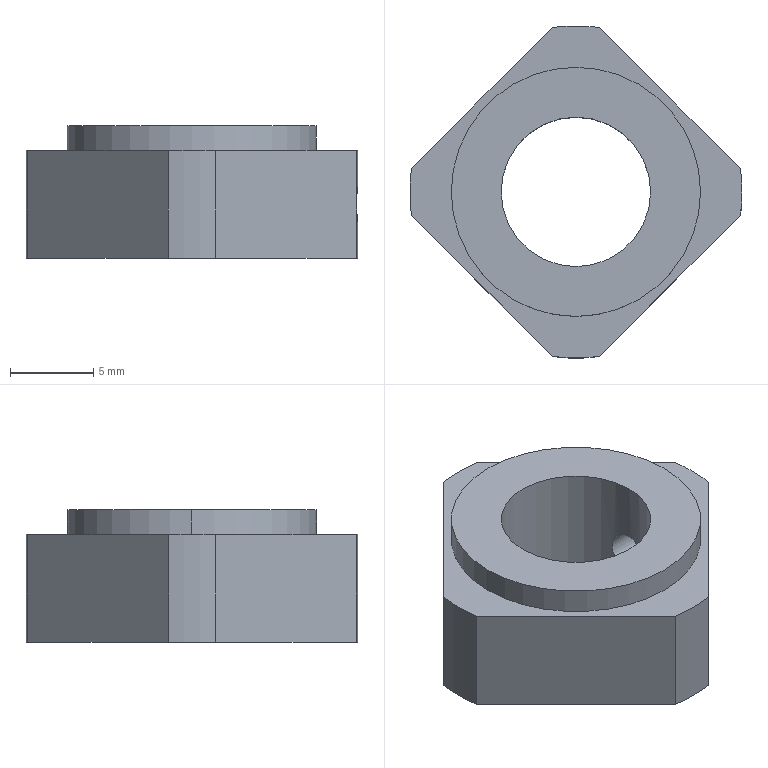Part | NX | features BREP 1 | 1 solid | 18 faces | box 20 x 20 x 8 mm | volume 1346 mm3 | cylinder 11 | plane 7 | commonest cylinder face diameters 20 x5 2.5 x2 9 x2 15 x2
STEP:
#1=CARTESIAN_POINT('',(4.5,0.,2.));
#2=VERTEX_POINT('',#1);
#3=CARTESIAN_POINT('',(10.,0.,2.));
#4=VERTEX_POINT('',#3);
#5=CARTESIAN_POINT('',(0.,0.,2.));
#6=DIRECTION('',(-1.,0.,0.));
#7=VECTOR('',#6,1000.);
#8=LINE('',#5,#7);
#9=EDGE_CURVE('',#2,#4,#8,.F.);
#10=ORIENTED_EDGE('',*,*,#9,.T.);
#11=CARTESIAN_POINT('',(10.,0.,4.5));
#12=VERTEX_POINT('',#11);
#13=CARTESIAN_POINT('',(10.,0.,2.));
#14=CARTESIAN_POINT('',(10.,0.1547,2.));
#15=CARTESIAN_POINT('',(9.992,0.4424,2.068));
#16=CARTESIAN_POINT('',(9.979,0.6457,2.172));
#17=CARTESIAN_POINT('',(9.961,0.894,2.354));
#18=CARTESIAN_POINT('',(9.942,1.078,2.604));
#19=CARTESIAN_POINT('',(9.93,1.181,2.81));
#20=CARTESIAN_POINT('',(9.916,1.296,3.249));
#21=CARTESIAN_POINT('',(9.93,1.182,3.688));
#22=CARTESIAN_POINT('',(9.942,1.079,3.895));
#23=CARTESIAN_POINT('',(9.961,0.8953,4.144));
#24=CARTESIAN_POINT('',(9.979,0.6468,4.327));
#25=CARTESIAN_POINT('',(9.992,0.4446,4.431));
#26=CARTESIAN_POINT('',(10.,0.1552,4.5));
#27=CARTESIAN_POINT('',(10.,0.,4.5));
#28=B_SPLINE_CURVE_WITH_KNOTS('',3,(#13,#14,#15,#16,#17,#18,#19,#20,#21,#22,#23,#24,#25,#26,#27),.UNSPECIFIED.,.F.,.F.,(4,1,1,1,1,1,1,1,1,1,1,1,4),(0.,0.125,0.1875,0.25,0.3125,0.375,0.5,0.625,0.6875,0.75,0.8125,0.875,1.),.UNSPECIFIED.);
#29=EDGE_CURVE('',#4,#12,#28,.T.);
#30=ORIENTED_EDGE('',*,*,#29,.T.);
#31=CARTESIAN_POINT('',(4.5,0.,4.5));
#32=VERTEX_POINT('',#31);
#33=CARTESIAN_POINT('',(0.,0.,4.5));
#34=DIRECTION('',(-1.,0.,0.));
#35=VECTOR('',#34,1000.);
#36=LINE('',#33,#35);
#37=EDGE_CURVE('',#32,#12,#36,.F.);
#38=ORIENTED_EDGE('',*,*,#37,.F.);
#39=CARTESIAN_POINT('',(4.5,0.,4.5));
#40=CARTESIAN_POINT('',(4.5,0.1559,4.5));
#41=CARTESIAN_POINT('',(4.481,0.4441,4.432));
#42=CARTESIAN_POINT('',(4.454,0.65,4.325));
#43=CARTESIAN_POINT('',(4.413,0.8939,4.146));
#44=CARTESIAN_POINT('',(4.37,1.08,3.893));
#45=CARTESIAN_POINT('',(4.343,1.18,3.692));
#46=CARTESIAN_POINT('',(4.31,1.297,3.25));
#47=CARTESIAN_POINT('',(4.343,1.179,2.807));
#48=CARTESIAN_POINT('',(4.37,1.08,2.607));
#49=CARTESIAN_POINT('',(4.413,0.8931,2.353));
#50=CARTESIAN_POINT('',(4.454,0.6493,2.175));
#51=CARTESIAN_POINT('',(4.482,0.4423,2.067));
#52=CARTESIAN_POINT('',(4.5,0.1555,2.));
#53=CARTESIAN_POINT('',(4.5,0.,2.));
#54=B_SPLINE_CURVE_WITH_KNOTS('',3,(#39,#40,#41,#42,#43,#44,#45,#46,#47,#48,#49,#50,#51,#52,#53),.UNSPECIFIED.,.F.,.F.,(4,1,1,1,1,1,1,1,1,1,1,1,4),(0.,0.125,0.1875,0.25,0.3125,0.375,0.5,0.625,0.6875,0.75,0.8125,0.875,1.),.UNSPECIFIED.);
#55=EDGE_CURVE('',#2,#32,#54,.F.);
#56=ORIENTED_EDGE('',*,*,#55,.F.);
#57=EDGE_LOOP('',(#10,#30,#38,#56));
#58=FACE_BOUND('',#57,.T.);
#59=CARTESIAN_POINT('',(0.,0.,3.25));
#60=DIRECTION('',(-1.,0.,0.));
#61=DIRECTION('',(0.,0.,1.));
#62=AXIS2_PLACEMENT_3D('',#59,#60,#61);
#63=CYLINDRICAL_SURFACE('',#62,1.25);
#64=ADVANCED_FACE('',(#58),#63,.F.);
#65=CARTESIAN_POINT('',(4.5,0.,8.));
#66=VERTEX_POINT('',#65);
#67=CARTESIAN_POINT('',(4.5,0.,0.));
#68=DIRECTION('',(0.,0.,-1.));
#69=VECTOR('',#68,1000.);
#70=LINE('',#67,#69);
#71=EDGE_CURVE('',#66,#32,#70,.T.);
#72=ORIENTED_EDGE('',*,*,#71,.F.);
#73=CARTESIAN_POINT('',(-4.5,0.,8.));
#74=VERTEX_POINT('',#73);
#75=CARTESIAN_POINT('',(0.,0.,8.));
#76=DIRECTION('',(0.,0.,-1.));
#77=DIRECTION('',(-1.,0.,0.));
#78=AXIS2_PLACEMENT_3D('',#75,#76,#77);
#79=CIRCLE('',#78,4.5);
#80=EDGE_CURVE('',#74,#66,#79,.T.);
#81=ORIENTED_EDGE('',*,*,#80,.F.);
#82=CARTESIAN_POINT('',(-4.5,0.,0.));
#83=VERTEX_POINT('',#82);
#84=CARTESIAN_POINT('',(-4.5,0.,0.));
#85=DIRECTION('',(0.,0.,-1.));
#86=VECTOR('',#85,1000.);
#87=LINE('',#84,#86);
#88=EDGE_CURVE('',#74,#83,#87,.T.);
#89=ORIENTED_EDGE('',*,*,#88,.T.);
#90=CARTESIAN_POINT('',(4.5,0.,0.));
#91=VERTEX_POINT('',#90);
#92=CARTESIAN_POINT('',(0.,0.,0.));
#93=DIRECTION('',(0.,0.,-1.));
#94=DIRECTION('',(-1.,0.,0.));
#95=AXIS2_PLACEMENT_3D('',#92,#93,#94);
#96=CIRCLE('',#95,4.5);
#97=EDGE_CURVE('',#83,#91,#96,.T.);
#98=ORIENTED_EDGE('',*,*,#97,.T.);
#99=CARTESIAN_POINT('',(4.5,0.,0.));
#100=DIRECTION('',(0.,0.,-1.));
#101=VECTOR('',#100,1000.);
#102=LINE('',#99,#101);
#103=EDGE_CURVE('',#2,#91,#102,.T.);
#104=ORIENTED_EDGE('',*,*,#103,.F.);
#105=ORIENTED_EDGE('',*,*,#55,.T.);
#106=EDGE_LOOP('',(#72,#81,#89,#98,#104,#105));
#107=FACE_BOUND('',#106,.T.);
#108=CARTESIAN_POINT('',(0.,0.,0.));
#109=DIRECTION('',(0.,0.,-1.));
#110=DIRECTION('',(-1.,0.,0.));
#111=AXIS2_PLACEMENT_3D('',#108,#109,#110);
#112=CYLINDRICAL_SURFACE('',#111,4.5);
#113=ADVANCED_FACE('',(#107),#112,.F.);
#114=CARTESIAN_POINT('',(-7.5,0.,8.));
#115=VERTEX_POINT('',#114);
#116=CARTESIAN_POINT('',(-7.5,0.,6.5));
#117=VERTEX_POINT('',#116);
#118=CARTESIAN_POINT('',(-7.5,0.,6.5));
#119=DIRECTION('',(0.,0.,1.));
#120=VECTOR('',#119,1000.);
#121=LINE('',#118,#120);
#122=EDGE_CURVE('',#115,#117,#121,.F.);
#123=ORIENTED_EDGE('',*,*,#122,.T.);
#124=CARTESIAN_POINT('',(7.5,0.,6.5));
#125=VERTEX_POINT('',#124);
#126=CARTESIAN_POINT('',(0.,0.,6.5));
#127=DIRECTION('',(0.,0.,1.));
#128=DIRECTION('',(1.,0.,0.));
#129=AXIS2_PLACEMENT_3D('',#126,#127,#128);
#130=CIRCLE('',#129,7.5);
#131=EDGE_CURVE('',#117,#125,#130,.T.);
#132=ORIENTED_EDGE('',*,*,#131,.T.);
#133=CARTESIAN_POINT('',(7.5,0.,8.));
#134=VERTEX_POINT('',#133);
#135=CARTESIAN_POINT('',(7.5,0.,6.5));
#136=DIRECTION('',(0.,0.,1.));
#137=VECTOR('',#136,1000.);
#138=LINE('',#135,#137);
#139=EDGE_CURVE('',#134,#125,#138,.F.);
#140=ORIENTED_EDGE('',*,*,#139,.F.);
#141=CARTESIAN_POINT('',(0.,0.,8.));
#142=DIRECTION('',(0.,0.,1.));
#143=DIRECTION('',(1.,0.,0.));
#144=AXIS2_PLACEMENT_3D('',#141,#142,#143);
#145=CIRCLE('',#144,7.5);
#146=EDGE_CURVE('',#115,#134,#145,.T.);
#147=ORIENTED_EDGE('',*,*,#146,.F.);
#148=EDGE_LOOP('',(#123,#132,#140,#147));
#149=FACE_BOUND('',#148,.T.);
#150=CARTESIAN_POINT('',(0.,0.,6.5));
#151=DIRECTION('',(0.,0.,1.));
#152=DIRECTION('',(1.,0.,0.));
#153=AXIS2_PLACEMENT_3D('',#150,#151,#152);
#154=CYLINDRICAL_SURFACE('',#153,7.5);
#155=ADVANCED_FACE('',(#149),#154,.T.);
#156=CARTESIAN_POINT('',(0.,0.,6.5));
#157=DIRECTION('',(0.,0.,1.));
#158=DIRECTION('',(1.,0.,0.));
#159=AXIS2_PLACEMENT_3D('',#156,#157,#158);
#160=CIRCLE('',#159,7.5);
#161=EDGE_CURVE('',#125,#117,#160,.T.);
#162=ORIENTED_EDGE('',*,*,#161,.F.);
#163=ORIENTED_EDGE('',*,*,#131,.F.);
#164=EDGE_LOOP('',(#162,#163));
#165=FACE_BOUND('',#164,.T.);
#166=CARTESIAN_POINT('',(-1.414,9.899,6.5));
#167=VERTEX_POINT('',#166);
#168=CARTESIAN_POINT('',(-9.899,1.414,6.5));
#169=VERTEX_POINT('',#168);
#170=CARTESIAN_POINT('',(-11.314,0.,6.5));
#171=DIRECTION('',(-0.7071,-0.7071,0.));
#172=VECTOR('',#171,1000.);
#173=LINE('',#170,#172);
#174=EDGE_CURVE('',#167,#169,#173,.T.);
#175=ORIENTED_EDGE('',*,*,#174,.T.);
#176=CARTESIAN_POINT('',(-9.899,-1.414,6.5));
#177=VERTEX_POINT('',#176);
#178=CARTESIAN_POINT('',(0.,0.,6.5));
#179=DIRECTION('',(0.,0.,-1.));
#180=DIRECTION('',(1.,0.,0.));
#181=AXIS2_PLACEMENT_3D('',#178,#179,#180);
#182=CIRCLE('',#181,10.);
#183=EDGE_CURVE('',#177,#169,#182,.T.);
#184=ORIENTED_EDGE('',*,*,#183,.F.);
#185=CARTESIAN_POINT('',(-1.414,-9.899,6.5));
#186=VERTEX_POINT('',#185);
#187=CARTESIAN_POINT('',(-11.314,0.,6.5));
#188=DIRECTION('',(0.7071,-0.7071,0.));
#189=VECTOR('',#188,1000.);
#190=LINE('',#187,#189);
#191=EDGE_CURVE('',#177,#186,#190,.T.);
#192=ORIENTED_EDGE('',*,*,#191,.T.);
#193=CARTESIAN_POINT('',(1.414,-9.899,6.5));
#194=VERTEX_POINT('',#193);
#195=CARTESIAN_POINT('',(0.,0.,6.5));
#196=DIRECTION('',(0.,0.,-1.));
#197=DIRECTION('',(1.,0.,0.));
#198=AXIS2_PLACEMENT_3D('',#195,#196,#197);
#199=CIRCLE('',#198,10.);
#200=EDGE_CURVE('',#194,#186,#199,.T.);
#201=ORIENTED_EDGE('',*,*,#200,.F.);
#202=CARTESIAN_POINT('',(9.899,-1.414,6.5));
#203=VERTEX_POINT('',#202);
#204=CARTESIAN_POINT('',(0.,-11.314,6.5));
#205=DIRECTION('',(0.7071,0.7071,0.));
#206=VECTOR('',#205,1000.);
#207=LINE('',#204,#206);
#208=EDGE_CURVE('',#194,#203,#207,.T.);
#209=ORIENTED_EDGE('',*,*,#208,.T.);
#210=CARTESIAN_POINT('',(10.,0.,6.5));
#211=VERTEX_POINT('',#210);
#212=CARTESIAN_POINT('',(0.,0.,6.5));
#213=DIRECTION('',(0.,0.,-1.));
#214=DIRECTION('',(1.,0.,0.));
#215=AXIS2_PLACEMENT_3D('',#212,#213,#214);
#216=CIRCLE('',#215,10.);
#217=EDGE_CURVE('',#211,#203,#216,.T.);
#218=ORIENTED_EDGE('',*,*,#217,.F.);
#219=CARTESIAN_POINT('',(9.899,1.414,6.5));
#220=VERTEX_POINT('',#219);
#221=CARTESIAN_POINT('',(0.,0.,6.5));
#222=DIRECTION('',(0.,0.,-1.));
#223=DIRECTION('',(1.,0.,0.));
#224=AXIS2_PLACEMENT_3D('',#221,#222,#223);
#225=CIRCLE('',#224,10.);
#226=EDGE_CURVE('',#220,#211,#225,.T.);
#227=ORIENTED_EDGE('',*,*,#226,.F.);
#228=CARTESIAN_POINT('',(1.414,9.899,6.5));
#229=VERTEX_POINT('',#228);
#230=CARTESIAN_POINT('',(0.,11.314,6.5));
#231=DIRECTION('',(-0.7071,0.7071,0.));
#232=VECTOR('',#231,1000.);
#233=LINE('',#230,#232);
#234=EDGE_CURVE('',#220,#229,#233,.T.);
#235=ORIENTED_EDGE('',*,*,#234,.T.);
#236=CARTESIAN_POINT('',(0.,0.,6.5));
#237=DIRECTION('',(0.,0.,-1.));
#238=DIRECTION('',(1.,0.,0.));
#239=AXIS2_PLACEMENT_3D('',#236,#237,#238);
#240=CIRCLE('',#239,10.);
#241=EDGE_CURVE('',#167,#229,#240,.T.);
#242=ORIENTED_EDGE('',*,*,#241,.F.);
#243=EDGE_LOOP('',(#175,#184,#192,#201,#209,#218,#227,#235,#242));
#244=FACE_BOUND('',#243,.T.);
#245=CARTESIAN_POINT('',(0.,0.,6.5));
#246=DIRECTION('',(0.,0.,1.));
#247=DIRECTION('',(1.,0.,0.));
#248=AXIS2_PLACEMENT_3D('',#245,#246,#247);
#249=PLANE('',#248);
#250=ADVANCED_FACE('',(#165,#244),#249,.T.);
#251=CARTESIAN_POINT('',(1.414,-9.899,0.));
#252=VERTEX_POINT('',#251);
#253=CARTESIAN_POINT('',(1.414,-9.899,-2.));
#254=DIRECTION('',(0.,0.,1.));
#255=VECTOR('',#254,1000.);
#256=LINE('',#253,#255);
#257=EDGE_CURVE('',#252,#194,#256,.T.);
#258=ORIENTED_EDGE('',*,*,#257,.T.);
#259=ORIENTED_EDGE('',*,*,#200,.T.);
#260=CARTESIAN_POINT('',(-1.414,-9.899,0.));
#261=VERTEX_POINT('',#260);
#262=CARTESIAN_POINT('',(-1.414,-9.899,-2.));
#263=DIRECTION('',(0.,0.,-1.));
#264=VECTOR('',#263,1000.);
#265=LINE('',#262,#264);
#266=EDGE_CURVE('',#186,#261,#265,.T.);
#267=ORIENTED_EDGE('',*,*,#266,.T.);
#268=CARTESIAN_POINT('',(0.,0.,0.));
#269=DIRECTION('',(0.,0.,1.));
#270=DIRECTION('',(1.,0.,0.));
#271=AXIS2_PLACEMENT_3D('',#268,#269,#270);
#272=CIRCLE('',#271,10.);
#273=EDGE_CURVE('',#261,#252,#272,.T.);
#274=ORIENTED_EDGE('',*,*,#273,.T.);
#275=EDGE_LOOP('',(#258,#259,#267,#274));
#276=FACE_BOUND('',#275,.T.);
#277=CARTESIAN_POINT('',(0.,0.,-2.));
#278=DIRECTION('',(0.,0.,1.));
#279=DIRECTION('',(1.,0.,0.));
#280=AXIS2_PLACEMENT_3D('',#277,#278,#279);
#281=CYLINDRICAL_SURFACE('',#280,10.);
#282=ADVANCED_FACE('',(#276),#281,.T.);
#283=CARTESIAN_POINT('',(10.,0.,0.));
#284=VERTEX_POINT('',#283);
#285=CARTESIAN_POINT('',(10.,0.,-2.));
#286=DIRECTION('',(0.,0.,1.));
#287=VECTOR('',#286,1000.);
#288=LINE('',#285,#287);
#289=EDGE_CURVE('',#284,#4,#288,.T.);
#290=ORIENTED_EDGE('',*,*,#289,.F.);
#291=CARTESIAN_POINT('',(9.899,1.414,0.));
#292=VERTEX_POINT('',#291);
#293=CARTESIAN_POINT('',(0.,0.,0.));
#294=DIRECTION('',(0.,0.,1.));
#295=DIRECTION('',(1.,0.,0.));
#296=AXIS2_PLACEMENT_3D('',#293,#294,#295);
#297=CIRCLE('',#296,10.);
#298=EDGE_CURVE('',#284,#292,#297,.T.);
#299=ORIENTED_EDGE('',*,*,#298,.T.);
#300=CARTESIAN_POINT('',(9.899,1.414,-2.));
#301=DIRECTION('',(0.,0.,1.));
#302=VECTOR('',#301,1000.);
#303=LINE('',#300,#302);
#304=EDGE_CURVE('',#292,#220,#303,.T.);
#305=ORIENTED_EDGE('',*,*,#304,.T.);
#306=ORIENTED_EDGE('',*,*,#226,.T.);
#307=CARTESIAN_POINT('',(10.,0.,-2.));
#308=DIRECTION('',(0.,0.,1.));
#309=VECTOR('',#308,1000.);
#310=LINE('',#307,#309);
#311=EDGE_CURVE('',#12,#211,#310,.T.);
#312=ORIENTED_EDGE('',*,*,#311,.F.);
#313=ORIENTED_EDGE('',*,*,#29,.F.);
#314=EDGE_LOOP('',(#290,#299,#305,#306,#312,#313));
#315=FACE_BOUND('',#314,.T.);
#316=CARTESIAN_POINT('',(0.,0.,-2.));
#317=DIRECTION('',(0.,0.,1.));
#318=DIRECTION('',(1.,0.,0.));
#319=AXIS2_PLACEMENT_3D('',#316,#317,#318);
#320=CYLINDRICAL_SURFACE('',#319,10.);
#321=ADVANCED_FACE('',(#315),#320,.T.);
#322=CARTESIAN_POINT('',(-1.414,9.899,0.));
#323=VERTEX_POINT('',#322);
#324=CARTESIAN_POINT('',(-1.414,9.899,-2.));
#325=DIRECTION('',(0.,0.,1.));
#326=VECTOR('',#325,1000.);
#327=LINE('',#324,#326);
#328=EDGE_CURVE('',#323,#167,#327,.T.);
#329=ORIENTED_EDGE('',*,*,#328,.T.);
#330=ORIENTED_EDGE('',*,*,#241,.T.);
#331=CARTESIAN_POINT('',(1.414,9.899,0.));
#332=VERTEX_POINT('',#331);
#333=CARTESIAN_POINT('',(1.414,9.899,-2.));
#334=DIRECTION('',(0.,0.,-1.));
#335=VECTOR('',#334,1000.);
#336=LINE('',#333,#335);
#337=EDGE_CURVE('',#229,#332,#336,.T.);
#338=ORIENTED_EDGE('',*,*,#337,.T.);
#339=CARTESIAN_POINT('',(0.,0.,0.));
#340=DIRECTION('',(0.,0.,1.));
#341=DIRECTION('',(1.,0.,0.));
#342=AXIS2_PLACEMENT_3D('',#339,#340,#341);
#343=CIRCLE('',#342,10.);
#344=EDGE_CURVE('',#332,#323,#343,.T.);
#345=ORIENTED_EDGE('',*,*,#344,.T.);
#346=EDGE_LOOP('',(#329,#330,#338,#345));
#347=FACE_BOUND('',#346,.T.);
#348=CARTESIAN_POINT('',(0.,0.,-2.));
#349=DIRECTION('',(0.,0.,1.));
#350=DIRECTION('',(1.,0.,0.));
#351=AXIS2_PLACEMENT_3D('',#348,#349,#350);
#352=CYLINDRICAL_SURFACE('',#351,10.);
#353=ADVANCED_FACE('',(#347),#352,.T.);
#354=CARTESIAN_POINT('',(-9.899,-1.414,0.));
#355=VERTEX_POINT('',#354);
#356=CARTESIAN_POINT('',(-9.899,-1.414,-2.));
#357=DIRECTION('',(0.,0.,1.));
#358=VECTOR('',#357,1000.);
#359=LINE('',#356,#358);
#360=EDGE_CURVE('',#355,#177,#359,.T.);
#361=ORIENTED_EDGE('',*,*,#360,.T.);
#362=ORIENTED_EDGE('',*,*,#183,.T.);
#363=CARTESIAN_POINT('',(-9.899,1.414,0.));
#364=VERTEX_POINT('',#363);
#365=CARTESIAN_POINT('',(-9.899,1.414,-2.));
#366=DIRECTION('',(0.,0.,-1.));
#367=VECTOR('',#366,1000.);
#368=LINE('',#365,#367);
#369=EDGE_CURVE('',#169,#364,#368,.T.);
#370=ORIENTED_EDGE('',*,*,#369,.T.);
#371=CARTESIAN_POINT('',(0.,0.,0.));
#372=DIRECTION('',(0.,0.,1.));
#373=DIRECTION('',(1.,0.,0.));
#374=AXIS2_PLACEMENT_3D('',#371,#372,#373);
#375=CIRCLE('',#374,10.);
#376=EDGE_CURVE('',#364,#355,#375,.T.);
#377=ORIENTED_EDGE('',*,*,#376,.T.);
#378=EDGE_LOOP('',(#361,#362,#370,#377));
#379=FACE_BOUND('',#378,.T.);
#380=CARTESIAN_POINT('',(0.,0.,-2.));
#381=DIRECTION('',(0.,0.,1.));
#382=DIRECTION('',(1.,0.,0.));
#383=AXIS2_PLACEMENT_3D('',#380,#381,#382);
#384=CYLINDRICAL_SURFACE('',#383,10.);
#385=ADVANCED_FACE('',(#379),#384,.T.);
#386=ORIENTED_EDGE('',*,*,#174,.F.);
#387=ORIENTED_EDGE('',*,*,#328,.F.);
#388=CARTESIAN_POINT('',(-11.314,0.,0.));
#389=DIRECTION('',(-0.7071,-0.7071,0.));
#390=VECTOR('',#389,1000.);
#391=LINE('',#388,#390);
#392=EDGE_CURVE('',#323,#364,#391,.T.);
#393=ORIENTED_EDGE('',*,*,#392,.T.);
#394=ORIENTED_EDGE('',*,*,#369,.F.);
#395=EDGE_LOOP('',(#386,#387,#393,#394));
#396=FACE_BOUND('',#395,.T.);
#397=CARTESIAN_POINT('',(-11.314,0.,8.));
#398=DIRECTION('',(0.7071,-0.7071,0.));
#399=DIRECTION('',(0.7071,0.7071,0.));
#400=AXIS2_PLACEMENT_3D('',#397,#398,#399);
#401=PLANE('',#400);
#402=ADVANCED_FACE('',(#396),#401,.F.);
#403=ORIENTED_EDGE('',*,*,#234,.F.);
#404=ORIENTED_EDGE('',*,*,#304,.F.);
#405=CARTESIAN_POINT('',(0.,11.314,0.));
#406=DIRECTION('',(-0.7071,0.7071,0.));
#407=VECTOR('',#406,1000.);
#408=LINE('',#405,#407);
#409=EDGE_CURVE('',#292,#332,#408,.T.);
#410=ORIENTED_EDGE('',*,*,#409,.T.);
#411=ORIENTED_EDGE('',*,*,#337,.F.);
#412=EDGE_LOOP('',(#403,#404,#410,#411));
#413=FACE_BOUND('',#412,.T.);
#414=CARTESIAN_POINT('',(0.,11.314,8.));
#415=DIRECTION('',(-0.7071,-0.7071,0.));
#416=DIRECTION('',(0.7071,-0.7071,0.));
#417=AXIS2_PLACEMENT_3D('',#414,#415,#416);
#418=PLANE('',#417);
#419=ADVANCED_FACE('',(#413),#418,.F.);
#420=ORIENTED_EDGE('',*,*,#208,.F.);
#421=ORIENTED_EDGE('',*,*,#257,.F.);
#422=CARTESIAN_POINT('',(9.899,-1.414,0.));
#423=VERTEX_POINT('',#422);
#424=CARTESIAN_POINT('',(0.,-11.314,0.));
#425=DIRECTION('',(0.7071,0.7071,0.));
#426=VECTOR('',#425,1000.);
#427=LINE('',#424,#426);
#428=EDGE_CURVE('',#252,#423,#427,.T.);
#429=ORIENTED_EDGE('',*,*,#428,.T.);
#430=CARTESIAN_POINT('',(9.899,-1.414,-2.));
#431=DIRECTION('',(0.,0.,-1.));
#432=VECTOR('',#431,1000.);
#433=LINE('',#430,#432);
#434=EDGE_CURVE('',#203,#423,#433,.T.);
#435=ORIENTED_EDGE('',*,*,#434,.F.);
#436=EDGE_LOOP('',(#420,#421,#429,#435));
#437=FACE_BOUND('',#436,.T.);
#438=CARTESIAN_POINT('',(0.,-11.314,8.));
#439=DIRECTION('',(-0.7071,0.7071,0.));
#440=DIRECTION('',(-0.7071,-0.7071,0.));
#441=AXIS2_PLACEMENT_3D('',#438,#439,#440);
#442=PLANE('',#441);
#443=ADVANCED_FACE('',(#437),#442,.F.);
#444=ORIENTED_EDGE('',*,*,#191,.F.);
#445=ORIENTED_EDGE('',*,*,#360,.F.);
#446=CARTESIAN_POINT('',(-11.314,0.,0.));
#447=DIRECTION('',(0.7071,-0.7071,0.));
#448=VECTOR('',#447,1000.);
#449=LINE('',#446,#448);
#450=EDGE_CURVE('',#355,#261,#449,.T.);
#451=ORIENTED_EDGE('',*,*,#450,.T.);
#452=ORIENTED_EDGE('',*,*,#266,.F.);
#453=EDGE_LOOP('',(#444,#445,#451,#452));
#454=FACE_BOUND('',#453,.T.);
#455=CARTESIAN_POINT('',(-11.314,0.,8.));
#456=DIRECTION('',(0.7071,0.7071,0.));
#457=DIRECTION('',(-0.7071,0.7071,0.));
#458=AXIS2_PLACEMENT_3D('',#455,#456,#457);
#459=PLANE('',#458);
#460=ADVANCED_FACE('',(#454),#459,.F.);
#461=CARTESIAN_POINT('',(0.,0.,8.));
#462=DIRECTION('',(0.,0.,1.));
#463=DIRECTION('',(1.,0.,0.));
#464=AXIS2_PLACEMENT_3D('',#461,#462,#463);
#465=CIRCLE('',#464,7.5);
#466=EDGE_CURVE('',#134,#115,#465,.T.);
#467=ORIENTED_EDGE('',*,*,#466,.T.);
#468=ORIENTED_EDGE('',*,*,#146,.T.);
#469=EDGE_LOOP('',(#467,#468));
#470=FACE_BOUND('',#469,.T.);
#471=ORIENTED_EDGE('',*,*,#80,.T.);
#472=CARTESIAN_POINT('',(0.,0.,8.));
#473=DIRECTION('',(0.,0.,-1.));
#474=DIRECTION('',(-1.,0.,0.));
#475=AXIS2_PLACEMENT_3D('',#472,#473,#474);
#476=CIRCLE('',#475,4.5);
#477=EDGE_CURVE('',#66,#74,#476,.T.);
#478=ORIENTED_EDGE('',*,*,#477,.T.);
#479=EDGE_LOOP('',(#471,#478));
#480=FACE_BOUND('',#479,.T.);
#481=CARTESIAN_POINT('',(0.,0.,8.));
#482=DIRECTION('',(0.,0.,1.));
#483=DIRECTION('',(1.,0.,0.));
#484=AXIS2_PLACEMENT_3D('',#481,#482,#483);
#485=PLANE('',#484);
#486=ADVANCED_FACE('',(#470,#480),#485,.T.);
#487=ORIENTED_EDGE('',*,*,#97,.F.);
#488=CARTESIAN_POINT('',(0.,0.,0.));
#489=DIRECTION('',(0.,0.,-1.));
#490=DIRECTION('',(-1.,0.,0.));
#491=AXIS2_PLACEMENT_3D('',#488,#489,#490);
#492=CIRCLE('',#491,4.5);
#493=EDGE_CURVE('',#91,#83,#492,.T.);
#494=ORIENTED_EDGE('',*,*,#493,.F.);
#495=EDGE_LOOP('',(#487,#494));
#496=FACE_BOUND('',#495,.T.);
#497=ORIENTED_EDGE('',*,*,#344,.F.);
#498=ORIENTED_EDGE('',*,*,#409,.F.);
#499=ORIENTED_EDGE('',*,*,#298,.F.);
#500=CARTESIAN_POINT('',(0.,0.,0.));
#501=DIRECTION('',(0.,0.,1.));
#502=DIRECTION('',(1.,0.,0.));
#503=AXIS2_PLACEMENT_3D('',#500,#501,#502);
#504=CIRCLE('',#503,10.);
#505=EDGE_CURVE('',#423,#284,#504,.T.);
#506=ORIENTED_EDGE('',*,*,#505,.F.);
#507=ORIENTED_EDGE('',*,*,#428,.F.);
#508=ORIENTED_EDGE('',*,*,#273,.F.);
#509=ORIENTED_EDGE('',*,*,#450,.F.);
#510=ORIENTED_EDGE('',*,*,#376,.F.);
#511=ORIENTED_EDGE('',*,*,#392,.F.);
#512=EDGE_LOOP('',(#497,#498,#499,#506,#507,#508,#509,#510,#511));
#513=FACE_BOUND('',#512,.T.);
#514=CARTESIAN_POINT('',(0.,0.,0.));
#515=DIRECTION('',(0.,0.,1.));
#516=DIRECTION('',(1.,0.,0.));
#517=AXIS2_PLACEMENT_3D('',#514,#515,#516);
#518=PLANE('',#517);
#519=ADVANCED_FACE('',(#496,#513),#518,.F.);
#520=ORIENTED_EDGE('',*,*,#505,.T.);
#521=ORIENTED_EDGE('',*,*,#289,.T.);
#522=CARTESIAN_POINT('',(10.,0.,2.));
#523=CARTESIAN_POINT('',(10.,-0.3315,2.));
#524=CARTESIAN_POINT('',(9.961,-0.9772,2.27));
#525=CARTESIAN_POINT('',(9.902,-1.386,3.251));
#526=CARTESIAN_POINT('',(9.961,-0.9772,4.229));
#527=CARTESIAN_POINT('',(10.,-0.3319,4.5));
#528=CARTESIAN_POINT('',(10.,0.,4.5));
#529=B_SPLINE_CURVE_WITH_KNOTS('',3,(#522,#523,#524,#525,#526,#527,#528),.UNSPECIFIED.,.F.,.F.,(4,1,1,1,4),(0.,0.25,0.5,0.75,1.),.UNSPECIFIED.);
#530=EDGE_CURVE('',#12,#4,#529,.F.);
#531=ORIENTED_EDGE('',*,*,#530,.F.);
#532=ORIENTED_EDGE('',*,*,#311,.T.);
#533=ORIENTED_EDGE('',*,*,#217,.T.);
#534=ORIENTED_EDGE('',*,*,#434,.T.);
#535=EDGE_LOOP('',(#520,#521,#531,#532,#533,#534));
#536=FACE_BOUND('',#535,.T.);
#537=CARTESIAN_POINT('',(0.,0.,-2.));
#538=DIRECTION('',(0.,0.,1.));
#539=DIRECTION('',(1.,0.,0.));
#540=AXIS2_PLACEMENT_3D('',#537,#538,#539);
#541=CYLINDRICAL_SURFACE('',#540,10.);
#542=ADVANCED_FACE('',(#536),#541,.T.);
#543=ORIENTED_EDGE('',*,*,#161,.T.);
#544=ORIENTED_EDGE('',*,*,#122,.F.);
#545=ORIENTED_EDGE('',*,*,#466,.F.);
#546=ORIENTED_EDGE('',*,*,#139,.T.);
#547=EDGE_LOOP('',(#543,#544,#545,#546));
#548=FACE_BOUND('',#547,.T.);
#549=CARTESIAN_POINT('',(0.,0.,6.5));
#550=DIRECTION('',(0.,0.,1.));
#551=DIRECTION('',(1.,0.,0.));
#552=AXIS2_PLACEMENT_3D('',#549,#550,#551);
#553=CYLINDRICAL_SURFACE('',#552,7.5);
#554=ADVANCED_FACE('',(#548),#553,.T.);
#555=ORIENTED_EDGE('',*,*,#477,.F.);
#556=ORIENTED_EDGE('',*,*,#71,.T.);
#557=CARTESIAN_POINT('',(4.5,0.,4.5));
#558=CARTESIAN_POINT('',(4.5,-0.3323,4.5));
#559=CARTESIAN_POINT('',(4.413,-0.9772,4.229));
#560=CARTESIAN_POINT('',(4.278,-1.387,3.251));
#561=CARTESIAN_POINT('',(4.413,-0.9764,2.27));
#562=CARTESIAN_POINT('',(4.5,-0.3318,2.));
#563=CARTESIAN_POINT('',(4.5,0.,2.));
#564=B_SPLINE_CURVE_WITH_KNOTS('',3,(#557,#558,#559,#560,#561,#562,#563),.UNSPECIFIED.,.F.,.F.,(4,1,1,1,4),(0.,0.25,0.5,0.75,1.),.UNSPECIFIED.);
#565=EDGE_CURVE('',#32,#2,#564,.T.);
#566=ORIENTED_EDGE('',*,*,#565,.T.);
#567=ORIENTED_EDGE('',*,*,#103,.T.);
#568=ORIENTED_EDGE('',*,*,#493,.T.);
#569=ORIENTED_EDGE('',*,*,#88,.F.);
#570=EDGE_LOOP('',(#555,#556,#566,#567,#568,#569));
#571=FACE_BOUND('',#570,.T.);
#572=CARTESIAN_POINT('',(0.,0.,0.));
#573=DIRECTION('',(0.,0.,-1.));
#574=DIRECTION('',(-1.,0.,0.));
#575=AXIS2_PLACEMENT_3D('',#572,#573,#574);
#576=CYLINDRICAL_SURFACE('',#575,4.5);
#577=ADVANCED_FACE('',(#571),#576,.F.);
#578=ORIENTED_EDGE('',*,*,#530,.T.);
#579=ORIENTED_EDGE('',*,*,#9,.F.);
#580=ORIENTED_EDGE('',*,*,#565,.F.);
#581=ORIENTED_EDGE('',*,*,#37,.T.);
#582=EDGE_LOOP('',(#578,#579,#580,#581));
#583=FACE_BOUND('',#582,.T.);
#584=CARTESIAN_POINT('',(0.,0.,3.25));
#585=DIRECTION('',(-1.,0.,0.));
#586=DIRECTION('',(0.,0.,1.));
#587=AXIS2_PLACEMENT_3D('',#584,#585,#586);
#588=CYLINDRICAL_SURFACE('',#587,1.25);
#589=ADVANCED_FACE('',(#583),#588,.F.);
#590=CLOSED_SHELL('',(#64,#113,#155,#250,#282,#321,#353,#385,#402,#419,#443,#460,#486,#519,#542,#554,#577,#589));
#591=MANIFOLD_SOLID_BREP('',#590);
#592=(LENGTH_UNIT()NAMED_UNIT(*)SI_UNIT(.MILLI.,.METRE.));
#593=UNCERTAINTY_MEASURE_WITH_UNIT(LENGTH_MEASURE(0.0508),#592,'','');
#594=(NAMED_UNIT(*)PLANE_ANGLE_UNIT()SI_UNIT($,.RADIAN.));
#595=(NAMED_UNIT(*)SI_UNIT($,.STERADIAN.)SOLID_ANGLE_UNIT());
#596=(GEOMETRIC_REPRESENTATION_CONTEXT(3)GLOBAL_UNCERTAINTY_ASSIGNED_CONTEXT((#593))GLOBAL_UNIT_ASSIGNED_CONTEXT((#592,#594,#595))REPRESENTATION_CONTEXT('',''));
#597=ADVANCED_BREP_SHAPE_REPRESENTATION('',(#591),#596);